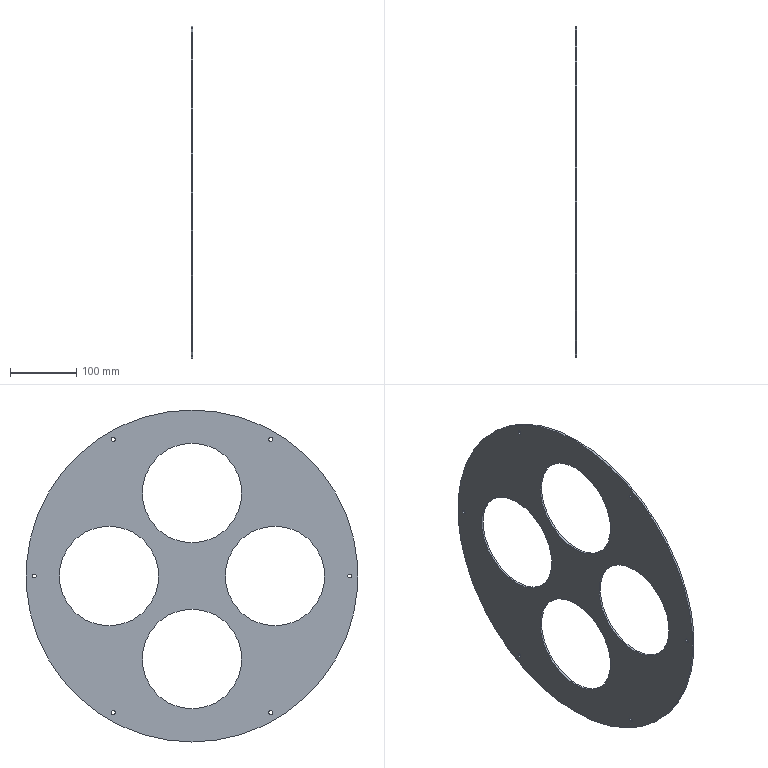Part | SolidWorks | features CirPattern 2, ICE 2, Extrusion 1 | 1 solid | 24 faces | box 3 x 500 x 500 mm | volume 376482 mm3 | cylinder 22 | plane 2 | commonest cylinder face diameters 6 x12 150 x8 500 x2
STEP:
#1=CARTESIAN_POINT('',(0.,118.75,208.681));
#2=VERTEX_POINT('',#1);
#3=CARTESIAN_POINT('',(0.,118.75,202.681));
#4=VERTEX_POINT('',#3);
#5=CARTESIAN_POINT('',(0.,118.75,205.681));
#6=DIRECTION('',(1.,0.,0.));
#7=DIRECTION('',(0.,0.,-1.));
#8=AXIS2_PLACEMENT_3D('',#5,#6,#7);
#9=CIRCLE('',#8,3.);
#10=EDGE_CURVE('',#2,#4,#9,.T.);
#11=ORIENTED_EDGE('',*,*,#10,.F.);
#12=CARTESIAN_POINT('',(3.,118.75,208.681));
#13=VERTEX_POINT('',#12);
#14=CARTESIAN_POINT('',(-17.,118.75,208.681));
#15=DIRECTION('',(1.,0.,0.));
#16=VECTOR('',#15,1000.);
#17=LINE('',#14,#16);
#18=EDGE_CURVE('',#2,#13,#17,.T.);
#19=ORIENTED_EDGE('',*,*,#18,.T.);
#20=CARTESIAN_POINT('',(3.,118.75,202.681));
#21=VERTEX_POINT('',#20);
#22=CARTESIAN_POINT('',(3.,118.75,205.681));
#23=DIRECTION('',(1.,0.,0.));
#24=DIRECTION('',(0.,-0.866,0.5));
#25=AXIS2_PLACEMENT_3D('',#22,#23,#24);
#26=CIRCLE('',#25,3.);
#27=EDGE_CURVE('',#13,#21,#26,.T.);
#28=ORIENTED_EDGE('',*,*,#27,.T.);
#29=CARTESIAN_POINT('',(-17.,118.75,202.681));
#30=DIRECTION('',(1.,0.,0.));
#31=VECTOR('',#30,1000.);
#32=LINE('',#29,#31);
#33=EDGE_CURVE('',#4,#21,#32,.T.);
#34=ORIENTED_EDGE('',*,*,#33,.F.);
#35=EDGE_LOOP('',(#11,#19,#28,#34));
#36=FACE_OUTER_BOUND('',#35,.T.);
#37=CARTESIAN_POINT('',(-17.,118.75,205.681));
#38=DIRECTION('',(1.,0.,0.));
#39=DIRECTION('',(0.,0.,-1.));
#40=AXIS2_PLACEMENT_3D('',#37,#38,#39);
#41=CYLINDRICAL_SURFACE('',#40,3.);
#42=ADVANCED_FACE('',(#36),#41,.F.);
#43=CARTESIAN_POINT('',(0.,237.5,3.));
#44=VERTEX_POINT('',#43);
#45=CARTESIAN_POINT('',(0.,237.5,-3.));
#46=VERTEX_POINT('',#45);
#47=CARTESIAN_POINT('',(0.,237.5,0.));
#48=DIRECTION('',(1.,0.,0.));
#49=DIRECTION('',(0.,0.,-1.));
#50=AXIS2_PLACEMENT_3D('',#47,#48,#49);
#51=CIRCLE('',#50,3.);
#52=EDGE_CURVE('',#44,#46,#51,.T.);
#53=ORIENTED_EDGE('',*,*,#52,.F.);
#54=CARTESIAN_POINT('',(3.,237.5,3.));
#55=VERTEX_POINT('',#54);
#56=CARTESIAN_POINT('',(-17.,237.5,3.));
#57=DIRECTION('',(1.,0.,0.));
#58=VECTOR('',#57,1000.);
#59=LINE('',#56,#58);
#60=EDGE_CURVE('',#44,#55,#59,.T.);
#61=ORIENTED_EDGE('',*,*,#60,.T.);
#62=CARTESIAN_POINT('',(3.,237.5,-3.));
#63=VERTEX_POINT('',#62);
#64=CARTESIAN_POINT('',(3.,237.5,0.));
#65=DIRECTION('',(1.,0.,0.));
#66=DIRECTION('',(0.,0.,1.));
#67=AXIS2_PLACEMENT_3D('',#64,#65,#66);
#68=CIRCLE('',#67,3.);
#69=EDGE_CURVE('',#55,#63,#68,.T.);
#70=ORIENTED_EDGE('',*,*,#69,.T.);
#71=CARTESIAN_POINT('',(-17.,237.5,-3.));
#72=DIRECTION('',(1.,0.,0.));
#73=VECTOR('',#72,1000.);
#74=LINE('',#71,#73);
#75=EDGE_CURVE('',#46,#63,#74,.T.);
#76=ORIENTED_EDGE('',*,*,#75,.F.);
#77=EDGE_LOOP('',(#53,#61,#70,#76));
#78=FACE_OUTER_BOUND('',#77,.T.);
#79=CARTESIAN_POINT('',(-17.,237.5,0.));
#80=DIRECTION('',(1.,0.,0.));
#81=DIRECTION('',(0.,0.,-1.));
#82=AXIS2_PLACEMENT_3D('',#79,#80,#81);
#83=CYLINDRICAL_SURFACE('',#82,3.);
#84=ADVANCED_FACE('',(#78),#83,.F.);
#85=CARTESIAN_POINT('',(0.,118.75,-202.681));
#86=VERTEX_POINT('',#85);
#87=CARTESIAN_POINT('',(0.,118.75,-208.681));
#88=VERTEX_POINT('',#87);
#89=CARTESIAN_POINT('',(0.,118.75,-205.681));
#90=DIRECTION('',(1.,0.,0.));
#91=DIRECTION('',(0.,0.,-1.));
#92=AXIS2_PLACEMENT_3D('',#89,#90,#91);
#93=CIRCLE('',#92,3.);
#94=EDGE_CURVE('',#86,#88,#93,.T.);
#95=ORIENTED_EDGE('',*,*,#94,.F.);
#96=CARTESIAN_POINT('',(3.,118.75,-202.681));
#97=VERTEX_POINT('',#96);
#98=CARTESIAN_POINT('',(-17.,118.75,-202.681));
#99=DIRECTION('',(1.,0.,0.));
#100=VECTOR('',#99,1000.);
#101=LINE('',#98,#100);
#102=EDGE_CURVE('',#86,#97,#101,.T.);
#103=ORIENTED_EDGE('',*,*,#102,.T.);
#104=CARTESIAN_POINT('',(3.,118.75,-208.681));
#105=VERTEX_POINT('',#104);
#106=CARTESIAN_POINT('',(3.,118.75,-205.681));
#107=DIRECTION('',(1.,0.,0.));
#108=DIRECTION('',(0.,0.866,0.5));
#109=AXIS2_PLACEMENT_3D('',#106,#107,#108);
#110=CIRCLE('',#109,3.);
#111=EDGE_CURVE('',#97,#105,#110,.T.);
#112=ORIENTED_EDGE('',*,*,#111,.T.);
#113=CARTESIAN_POINT('',(-17.,118.75,-208.681));
#114=DIRECTION('',(1.,0.,0.));
#115=VECTOR('',#114,1000.);
#116=LINE('',#113,#115);
#117=EDGE_CURVE('',#88,#105,#116,.T.);
#118=ORIENTED_EDGE('',*,*,#117,.F.);
#119=EDGE_LOOP('',(#95,#103,#112,#118));
#120=FACE_OUTER_BOUND('',#119,.T.);
#121=CARTESIAN_POINT('',(-17.,118.75,-205.681));
#122=DIRECTION('',(1.,0.,0.));
#123=DIRECTION('',(0.,0.,-1.));
#124=AXIS2_PLACEMENT_3D('',#121,#122,#123);
#125=CYLINDRICAL_SURFACE('',#124,3.);
#126=ADVANCED_FACE('',(#120),#125,.F.);
#127=CARTESIAN_POINT('',(0.,-118.75,-202.681));
#128=VERTEX_POINT('',#127);
#129=CARTESIAN_POINT('',(0.,-118.75,-208.681));
#130=VERTEX_POINT('',#129);
#131=CARTESIAN_POINT('',(0.,-118.75,-205.681));
#132=DIRECTION('',(1.,0.,0.));
#133=DIRECTION('',(0.,0.,-1.));
#134=AXIS2_PLACEMENT_3D('',#131,#132,#133);
#135=CIRCLE('',#134,3.);
#136=EDGE_CURVE('',#128,#130,#135,.T.);
#137=ORIENTED_EDGE('',*,*,#136,.F.);
#138=CARTESIAN_POINT('',(3.,-118.75,-202.681));
#139=VERTEX_POINT('',#138);
#140=CARTESIAN_POINT('',(-17.,-118.75,-202.681));
#141=DIRECTION('',(1.,0.,0.));
#142=VECTOR('',#141,1000.);
#143=LINE('',#140,#142);
#144=EDGE_CURVE('',#128,#139,#143,.T.);
#145=ORIENTED_EDGE('',*,*,#144,.T.);
#146=CARTESIAN_POINT('',(3.,-118.75,-208.681));
#147=VERTEX_POINT('',#146);
#148=CARTESIAN_POINT('',(3.,-118.75,-205.681));
#149=DIRECTION('',(1.,0.,0.));
#150=DIRECTION('',(0.,0.866,-0.5));
#151=AXIS2_PLACEMENT_3D('',#148,#149,#150);
#152=CIRCLE('',#151,3.);
#153=EDGE_CURVE('',#139,#147,#152,.T.);
#154=ORIENTED_EDGE('',*,*,#153,.T.);
#155=CARTESIAN_POINT('',(-17.,-118.75,-208.681));
#156=DIRECTION('',(1.,0.,0.));
#157=VECTOR('',#156,1000.);
#158=LINE('',#155,#157);
#159=EDGE_CURVE('',#130,#147,#158,.T.);
#160=ORIENTED_EDGE('',*,*,#159,.F.);
#161=EDGE_LOOP('',(#137,#145,#154,#160));
#162=FACE_OUTER_BOUND('',#161,.T.);
#163=CARTESIAN_POINT('',(-17.,-118.75,-205.681));
#164=DIRECTION('',(1.,0.,0.));
#165=DIRECTION('',(0.,0.,-1.));
#166=AXIS2_PLACEMENT_3D('',#163,#164,#165);
#167=CYLINDRICAL_SURFACE('',#166,3.);
#168=ADVANCED_FACE('',(#162),#167,.F.);
#169=CARTESIAN_POINT('',(0.,-118.75,208.681));
#170=VERTEX_POINT('',#169);
#171=CARTESIAN_POINT('',(0.,-118.75,202.681));
#172=VERTEX_POINT('',#171);
#173=CARTESIAN_POINT('',(0.,-118.75,205.681));
#174=DIRECTION('',(1.,0.,0.));
#175=DIRECTION('',(0.,0.,-1.));
#176=AXIS2_PLACEMENT_3D('',#173,#174,#175);
#177=CIRCLE('',#176,3.);
#178=EDGE_CURVE('',#170,#172,#177,.T.);
#179=ORIENTED_EDGE('',*,*,#178,.F.);
#180=CARTESIAN_POINT('',(3.,-118.75,208.681));
#181=VERTEX_POINT('',#180);
#182=CARTESIAN_POINT('',(-17.,-118.75,208.681));
#183=DIRECTION('',(1.,0.,0.));
#184=VECTOR('',#183,1000.);
#185=LINE('',#182,#184);
#186=EDGE_CURVE('',#170,#181,#185,.T.);
#187=ORIENTED_EDGE('',*,*,#186,.T.);
#188=CARTESIAN_POINT('',(3.,-118.75,202.681));
#189=VERTEX_POINT('',#188);
#190=CARTESIAN_POINT('',(3.,-118.75,205.681));
#191=DIRECTION('',(1.,0.,0.));
#192=DIRECTION('',(0.,-0.866,-0.5));
#193=AXIS2_PLACEMENT_3D('',#190,#191,#192);
#194=CIRCLE('',#193,3.);
#195=EDGE_CURVE('',#181,#189,#194,.T.);
#196=ORIENTED_EDGE('',*,*,#195,.T.);
#197=CARTESIAN_POINT('',(-17.,-118.75,202.681));
#198=DIRECTION('',(1.,0.,0.));
#199=VECTOR('',#198,1000.);
#200=LINE('',#197,#199);
#201=EDGE_CURVE('',#172,#189,#200,.T.);
#202=ORIENTED_EDGE('',*,*,#201,.F.);
#203=EDGE_LOOP('',(#179,#187,#196,#202));
#204=FACE_OUTER_BOUND('',#203,.T.);
#205=CARTESIAN_POINT('',(-17.,-118.75,205.681));
#206=DIRECTION('',(1.,0.,0.));
#207=DIRECTION('',(0.,0.,-1.));
#208=AXIS2_PLACEMENT_3D('',#205,#206,#207);
#209=CYLINDRICAL_SURFACE('',#208,3.);
#210=ADVANCED_FACE('',(#204),#209,.F.);
#211=CARTESIAN_POINT('',(0.,-237.5,3.));
#212=VERTEX_POINT('',#211);
#213=CARTESIAN_POINT('',(0.,-237.5,-3.));
#214=VERTEX_POINT('',#213);
#215=CARTESIAN_POINT('',(0.,-237.5,0.));
#216=DIRECTION('',(1.,0.,0.));
#217=DIRECTION('',(0.,0.,-1.));
#218=AXIS2_PLACEMENT_3D('',#215,#216,#217);
#219=CIRCLE('',#218,3.);
#220=EDGE_CURVE('',#212,#214,#219,.T.);
#221=ORIENTED_EDGE('',*,*,#220,.F.);
#222=CARTESIAN_POINT('',(3.,-237.5,3.));
#223=VERTEX_POINT('',#222);
#224=CARTESIAN_POINT('',(-17.,-237.5,3.));
#225=DIRECTION('',(1.,0.,0.));
#226=VECTOR('',#225,1000.);
#227=LINE('',#224,#226);
#228=EDGE_CURVE('',#212,#223,#227,.T.);
#229=ORIENTED_EDGE('',*,*,#228,.T.);
#230=CARTESIAN_POINT('',(3.,-237.5,-3.));
#231=VERTEX_POINT('',#230);
#232=CARTESIAN_POINT('',(3.,-237.5,0.));
#233=DIRECTION('',(1.,0.,0.));
#234=DIRECTION('',(0.,0.,-1.));
#235=AXIS2_PLACEMENT_3D('',#232,#233,#234);
#236=CIRCLE('',#235,3.);
#237=EDGE_CURVE('',#223,#231,#236,.T.);
#238=ORIENTED_EDGE('',*,*,#237,.T.);
#239=CARTESIAN_POINT('',(-17.,-237.5,-3.));
#240=DIRECTION('',(1.,0.,0.));
#241=VECTOR('',#240,1000.);
#242=LINE('',#239,#241);
#243=EDGE_CURVE('',#214,#231,#242,.T.);
#244=ORIENTED_EDGE('',*,*,#243,.F.);
#245=EDGE_LOOP('',(#221,#229,#238,#244));
#246=FACE_OUTER_BOUND('',#245,.T.);
#247=CARTESIAN_POINT('',(-17.,-237.5,0.));
#248=DIRECTION('',(1.,0.,0.));
#249=DIRECTION('',(0.,0.,-1.));
#250=AXIS2_PLACEMENT_3D('',#247,#248,#249);
#251=CYLINDRICAL_SURFACE('',#250,3.);
#252=ADVANCED_FACE('',(#246),#251,.F.);
#253=CARTESIAN_POINT('',(0.,0.,-50.));
#254=VERTEX_POINT('',#253);
#255=CARTESIAN_POINT('',(0.,0.,-200.));
#256=VERTEX_POINT('',#255);
#257=CARTESIAN_POINT('',(0.,0.,-125.));
#258=DIRECTION('',(1.,0.,0.));
#259=DIRECTION('',(0.,0.,-1.));
#260=AXIS2_PLACEMENT_3D('',#257,#258,#259);
#261=CIRCLE('',#260,75.);
#262=EDGE_CURVE('',#254,#256,#261,.T.);
#263=ORIENTED_EDGE('',*,*,#262,.F.);
#264=CARTESIAN_POINT('',(3.,0.,-50.));
#265=VERTEX_POINT('',#264);
#266=CARTESIAN_POINT('',(-7.,0.,-50.));
#267=DIRECTION('',(1.,0.,0.));
#268=VECTOR('',#267,1000.);
#269=LINE('',#266,#268);
#270=EDGE_CURVE('',#254,#265,#269,.T.);
#271=ORIENTED_EDGE('',*,*,#270,.T.);
#272=CARTESIAN_POINT('',(3.,0.,-200.));
#273=VERTEX_POINT('',#272);
#274=CARTESIAN_POINT('',(3.,0.,-125.));
#275=DIRECTION('',(1.,0.,0.));
#276=DIRECTION('',(0.,-1.,0.));
#277=AXIS2_PLACEMENT_3D('',#274,#275,#276);
#278=CIRCLE('',#277,75.);
#279=EDGE_CURVE('',#265,#273,#278,.T.);
#280=ORIENTED_EDGE('',*,*,#279,.T.);
#281=CARTESIAN_POINT('',(-7.,0.,-200.));
#282=DIRECTION('',(1.,0.,0.));
#283=VECTOR('',#282,1000.);
#284=LINE('',#281,#283);
#285=EDGE_CURVE('',#256,#273,#284,.T.);
#286=ORIENTED_EDGE('',*,*,#285,.F.);
#287=EDGE_LOOP('',(#263,#271,#280,#286));
#288=FACE_OUTER_BOUND('',#287,.T.);
#289=CARTESIAN_POINT('',(-7.,0.,-125.));
#290=DIRECTION('',(1.,0.,0.));
#291=DIRECTION('',(0.,0.,-1.));
#292=AXIS2_PLACEMENT_3D('',#289,#290,#291);
#293=CYLINDRICAL_SURFACE('',#292,75.);
#294=ADVANCED_FACE('',(#288),#293,.F.);
#295=CARTESIAN_POINT('',(0.,-125.,75.));
#296=VERTEX_POINT('',#295);
#297=CARTESIAN_POINT('',(0.,-125.,-75.));
#298=VERTEX_POINT('',#297);
#299=CARTESIAN_POINT('',(0.,-125.,0.));
#300=DIRECTION('',(1.,0.,0.));
#301=DIRECTION('',(0.,0.,-1.));
#302=AXIS2_PLACEMENT_3D('',#299,#300,#301);
#303=CIRCLE('',#302,75.);
#304=EDGE_CURVE('',#296,#298,#303,.T.);
#305=ORIENTED_EDGE('',*,*,#304,.F.);
#306=CARTESIAN_POINT('',(3.,-125.,75.));
#307=VERTEX_POINT('',#306);
#308=CARTESIAN_POINT('',(-7.,-125.,75.));
#309=DIRECTION('',(1.,0.,0.));
#310=VECTOR('',#309,1000.);
#311=LINE('',#308,#310);
#312=EDGE_CURVE('',#296,#307,#311,.T.);
#313=ORIENTED_EDGE('',*,*,#312,.T.);
#314=CARTESIAN_POINT('',(3.,-125.,-75.));
#315=VERTEX_POINT('',#314);
#316=CARTESIAN_POINT('',(3.,-125.,0.));
#317=DIRECTION('',(1.,0.,0.));
#318=DIRECTION('',(0.,0.,1.));
#319=AXIS2_PLACEMENT_3D('',#316,#317,#318);
#320=CIRCLE('',#319,75.);
#321=EDGE_CURVE('',#307,#315,#320,.T.);
#322=ORIENTED_EDGE('',*,*,#321,.T.);
#323=CARTESIAN_POINT('',(-7.,-125.,-75.));
#324=DIRECTION('',(1.,0.,0.));
#325=VECTOR('',#324,1000.);
#326=LINE('',#323,#325);
#327=EDGE_CURVE('',#298,#315,#326,.T.);
#328=ORIENTED_EDGE('',*,*,#327,.F.);
#329=EDGE_LOOP('',(#305,#313,#322,#328));
#330=FACE_OUTER_BOUND('',#329,.T.);
#331=CARTESIAN_POINT('',(-7.,-125.,0.));
#332=DIRECTION('',(1.,0.,0.));
#333=DIRECTION('',(0.,0.,-1.));
#334=AXIS2_PLACEMENT_3D('',#331,#332,#333);
#335=CYLINDRICAL_SURFACE('',#334,75.);
#336=ADVANCED_FACE('',(#330),#335,.F.);
#337=CARTESIAN_POINT('',(0.,0.,200.));
#338=VERTEX_POINT('',#337);
#339=CARTESIAN_POINT('',(0.,0.,50.));
#340=VERTEX_POINT('',#339);
#341=CARTESIAN_POINT('',(0.,0.,125.));
#342=DIRECTION('',(1.,0.,0.));
#343=DIRECTION('',(0.,0.,-1.));
#344=AXIS2_PLACEMENT_3D('',#341,#342,#343);
#345=CIRCLE('',#344,75.);
#346=EDGE_CURVE('',#338,#340,#345,.T.);
#347=ORIENTED_EDGE('',*,*,#346,.F.);
#348=CARTESIAN_POINT('',(3.,0.,200.));
#349=VERTEX_POINT('',#348);
#350=CARTESIAN_POINT('',(-7.,0.,200.));
#351=DIRECTION('',(1.,0.,0.));
#352=VECTOR('',#351,1000.);
#353=LINE('',#350,#352);
#354=EDGE_CURVE('',#338,#349,#353,.T.);
#355=ORIENTED_EDGE('',*,*,#354,.T.);
#356=CARTESIAN_POINT('',(3.,0.,50.));
#357=VERTEX_POINT('',#356);
#358=CARTESIAN_POINT('',(3.,0.,125.));
#359=DIRECTION('',(1.,0.,0.));
#360=DIRECTION('',(0.,1.,0.));
#361=AXIS2_PLACEMENT_3D('',#358,#359,#360);
#362=CIRCLE('',#361,75.);
#363=EDGE_CURVE('',#349,#357,#362,.T.);
#364=ORIENTED_EDGE('',*,*,#363,.T.);
#365=CARTESIAN_POINT('',(-7.,0.,50.));
#366=DIRECTION('',(1.,0.,0.));
#367=VECTOR('',#366,1000.);
#368=LINE('',#365,#367);
#369=EDGE_CURVE('',#340,#357,#368,.T.);
#370=ORIENTED_EDGE('',*,*,#369,.F.);
#371=EDGE_LOOP('',(#347,#355,#364,#370));
#372=FACE_OUTER_BOUND('',#371,.T.);
#373=CARTESIAN_POINT('',(-7.,0.,125.));
#374=DIRECTION('',(1.,0.,0.));
#375=DIRECTION('',(0.,0.,-1.));
#376=AXIS2_PLACEMENT_3D('',#373,#374,#375);
#377=CYLINDRICAL_SURFACE('',#376,75.);
#378=ADVANCED_FACE('',(#372),#377,.F.);
#379=CARTESIAN_POINT('',(0.,125.,75.));
#380=VERTEX_POINT('',#379);
#381=CARTESIAN_POINT('',(0.,125.,-75.));
#382=VERTEX_POINT('',#381);
#383=CARTESIAN_POINT('',(0.,125.,0.));
#384=DIRECTION('',(1.,0.,0.));
#385=DIRECTION('',(0.,0.,-1.));
#386=AXIS2_PLACEMENT_3D('',#383,#384,#385);
#387=CIRCLE('',#386,75.);
#388=EDGE_CURVE('',#380,#382,#387,.T.);
#389=ORIENTED_EDGE('',*,*,#388,.F.);
#390=CARTESIAN_POINT('',(3.,125.,75.));
#391=VERTEX_POINT('',#390);
#392=CARTESIAN_POINT('',(-7.,125.,75.));
#393=DIRECTION('',(1.,0.,0.));
#394=VECTOR('',#393,1000.);
#395=LINE('',#392,#394);
#396=EDGE_CURVE('',#380,#391,#395,.T.);
#397=ORIENTED_EDGE('',*,*,#396,.T.);
#398=CARTESIAN_POINT('',(3.,125.,-75.));
#399=VERTEX_POINT('',#398);
#400=CARTESIAN_POINT('',(3.,125.,0.));
#401=DIRECTION('',(1.,0.,0.));
#402=DIRECTION('',(0.,0.,-1.));
#403=AXIS2_PLACEMENT_3D('',#400,#401,#402);
#404=CIRCLE('',#403,75.);
#405=EDGE_CURVE('',#391,#399,#404,.T.);
#406=ORIENTED_EDGE('',*,*,#405,.T.);
#407=CARTESIAN_POINT('',(-7.,125.,-75.));
#408=DIRECTION('',(1.,0.,0.));
#409=VECTOR('',#408,1000.);
#410=LINE('',#407,#409);
#411=EDGE_CURVE('',#382,#399,#410,.T.);
#412=ORIENTED_EDGE('',*,*,#411,.F.);
#413=EDGE_LOOP('',(#389,#397,#406,#412));
#414=FACE_OUTER_BOUND('',#413,.T.);
#415=CARTESIAN_POINT('',(-7.,125.,0.));
#416=DIRECTION('',(1.,0.,0.));
#417=DIRECTION('',(0.,0.,-1.));
#418=AXIS2_PLACEMENT_3D('',#415,#416,#417);
#419=CYLINDRICAL_SURFACE('',#418,75.);
#420=ADVANCED_FACE('',(#414),#419,.F.);
#421=CARTESIAN_POINT('',(3.,0.,-250.));
#422=VERTEX_POINT('',#421);
#423=CARTESIAN_POINT('',(3.,0.,250.));
#424=VERTEX_POINT('',#423);
#425=CARTESIAN_POINT('',(3.,0.,0.));
#426=DIRECTION('',(1.,0.,0.));
#427=DIRECTION('',(0.,0.,-1.));
#428=AXIS2_PLACEMENT_3D('',#425,#426,#427);
#429=CIRCLE('',#428,250.);
#430=EDGE_CURVE('',#422,#424,#429,.T.);
#431=ORIENTED_EDGE('',*,*,#430,.F.);
#432=CARTESIAN_POINT('',(0.,0.,-250.));
#433=VERTEX_POINT('',#432);
#434=CARTESIAN_POINT('',(3.,0.,-250.));
#435=DIRECTION('',(-1.,0.,0.));
#436=VECTOR('',#435,1000.);
#437=LINE('',#434,#436);
#438=EDGE_CURVE('',#422,#433,#437,.T.);
#439=ORIENTED_EDGE('',*,*,#438,.T.);
#440=CARTESIAN_POINT('',(0.,0.,250.));
#441=VERTEX_POINT('',#440);
#442=CARTESIAN_POINT('',(0.,0.,0.));
#443=DIRECTION('',(1.,0.,0.));
#444=DIRECTION('',(0.,0.,-1.));
#445=AXIS2_PLACEMENT_3D('',#442,#443,#444);
#446=CIRCLE('',#445,250.);
#447=EDGE_CURVE('',#433,#441,#446,.T.);
#448=ORIENTED_EDGE('',*,*,#447,.T.);
#449=CARTESIAN_POINT('',(3.,0.,250.));
#450=DIRECTION('',(-1.,0.,0.));
#451=VECTOR('',#450,1000.);
#452=LINE('',#449,#451);
#453=EDGE_CURVE('',#424,#441,#452,.T.);
#454=ORIENTED_EDGE('',*,*,#453,.F.);
#455=EDGE_LOOP('',(#431,#439,#448,#454));
#456=FACE_OUTER_BOUND('',#455,.T.);
#457=CARTESIAN_POINT('',(3.,0.,0.));
#458=DIRECTION('',(-1.,0.,0.));
#459=DIRECTION('',(0.,0.,1.));
#460=AXIS2_PLACEMENT_3D('',#457,#458,#459);
#461=CYLINDRICAL_SURFACE('',#460,250.);
#462=ADVANCED_FACE('',(#456),#461,.T.);
#463=ORIENTED_EDGE('',*,*,#438,.F.);
#464=CARTESIAN_POINT('',(3.,0.,0.));
#465=DIRECTION('',(1.,0.,0.));
#466=DIRECTION('',(0.,0.,-1.));
#467=AXIS2_PLACEMENT_3D('',#464,#465,#466);
#468=CIRCLE('',#467,250.);
#469=EDGE_CURVE('',#424,#422,#468,.T.);
#470=ORIENTED_EDGE('',*,*,#469,.F.);
#471=ORIENTED_EDGE('',*,*,#453,.T.);
#472=CARTESIAN_POINT('',(0.,0.,0.));
#473=DIRECTION('',(1.,0.,0.));
#474=DIRECTION('',(0.,0.,-1.));
#475=AXIS2_PLACEMENT_3D('',#472,#473,#474);
#476=CIRCLE('',#475,250.);
#477=EDGE_CURVE('',#441,#433,#476,.T.);
#478=ORIENTED_EDGE('',*,*,#477,.T.);
#479=EDGE_LOOP('',(#463,#470,#471,#478));
#480=FACE_OUTER_BOUND('',#479,.T.);
#481=CARTESIAN_POINT('',(3.,0.,0.));
#482=DIRECTION('',(-1.,0.,0.));
#483=DIRECTION('',(0.,0.,1.));
#484=AXIS2_PLACEMENT_3D('',#481,#482,#483);
#485=CYLINDRICAL_SURFACE('',#484,250.);
#486=ADVANCED_FACE('',(#480),#485,.T.);
#487=CARTESIAN_POINT('',(3.,118.75,205.681));
#488=DIRECTION('',(1.,0.,0.));
#489=DIRECTION('',(0.,-0.866,0.5));
#490=AXIS2_PLACEMENT_3D('',#487,#488,#489);
#491=CIRCLE('',#490,3.);
#492=EDGE_CURVE('',#21,#13,#491,.T.);
#493=ORIENTED_EDGE('',*,*,#492,.F.);
#494=ORIENTED_EDGE('',*,*,#27,.F.);
#495=EDGE_LOOP('',(#493,#494));
#496=FACE_BOUND('',#495,.T.);
#497=CARTESIAN_POINT('',(3.,237.5,0.));
#498=DIRECTION('',(1.,0.,0.));
#499=DIRECTION('',(0.,0.,1.));
#500=AXIS2_PLACEMENT_3D('',#497,#498,#499);
#501=CIRCLE('',#500,3.);
#502=EDGE_CURVE('',#63,#55,#501,.T.);
#503=ORIENTED_EDGE('',*,*,#502,.F.);
#504=ORIENTED_EDGE('',*,*,#69,.F.);
#505=EDGE_LOOP('',(#503,#504));
#506=FACE_BOUND('',#505,.T.);
#507=CARTESIAN_POINT('',(3.,118.75,-205.681));
#508=DIRECTION('',(1.,0.,0.));
#509=DIRECTION('',(0.,0.866,0.5));
#510=AXIS2_PLACEMENT_3D('',#507,#508,#509);
#511=CIRCLE('',#510,3.);
#512=EDGE_CURVE('',#105,#97,#511,.T.);
#513=ORIENTED_EDGE('',*,*,#512,.F.);
#514=ORIENTED_EDGE('',*,*,#111,.F.);
#515=EDGE_LOOP('',(#513,#514));
#516=FACE_BOUND('',#515,.T.);
#517=CARTESIAN_POINT('',(3.,-118.75,-205.681));
#518=DIRECTION('',(1.,0.,0.));
#519=DIRECTION('',(0.,0.866,-0.5));
#520=AXIS2_PLACEMENT_3D('',#517,#518,#519);
#521=CIRCLE('',#520,3.);
#522=EDGE_CURVE('',#147,#139,#521,.T.);
#523=ORIENTED_EDGE('',*,*,#522,.F.);
#524=ORIENTED_EDGE('',*,*,#153,.F.);
#525=EDGE_LOOP('',(#523,#524));
#526=FACE_BOUND('',#525,.T.);
#527=CARTESIAN_POINT('',(3.,-118.75,205.681));
#528=DIRECTION('',(1.,0.,0.));
#529=DIRECTION('',(0.,-0.866,-0.5));
#530=AXIS2_PLACEMENT_3D('',#527,#528,#529);
#531=CIRCLE('',#530,3.);
#532=EDGE_CURVE('',#189,#181,#531,.T.);
#533=ORIENTED_EDGE('',*,*,#532,.F.);
#534=ORIENTED_EDGE('',*,*,#195,.F.);
#535=EDGE_LOOP('',(#533,#534));
#536=FACE_BOUND('',#535,.T.);
#537=CARTESIAN_POINT('',(3.,-237.5,0.));
#538=DIRECTION('',(1.,0.,0.));
#539=DIRECTION('',(0.,0.,-1.));
#540=AXIS2_PLACEMENT_3D('',#537,#538,#539);
#541=CIRCLE('',#540,3.);
#542=EDGE_CURVE('',#231,#223,#541,.T.);
#543=ORIENTED_EDGE('',*,*,#542,.F.);
#544=ORIENTED_EDGE('',*,*,#237,.F.);
#545=EDGE_LOOP('',(#543,#544));
#546=FACE_BOUND('',#545,.T.);
#547=CARTESIAN_POINT('',(3.,0.,-125.));
#548=DIRECTION('',(1.,0.,0.));
#549=DIRECTION('',(0.,-1.,0.));
#550=AXIS2_PLACEMENT_3D('',#547,#548,#549);
#551=CIRCLE('',#550,75.);
#552=EDGE_CURVE('',#273,#265,#551,.T.);
#553=ORIENTED_EDGE('',*,*,#552,.F.);
#554=ORIENTED_EDGE('',*,*,#279,.F.);
#555=EDGE_LOOP('',(#553,#554));
#556=FACE_BOUND('',#555,.T.);
#557=CARTESIAN_POINT('',(3.,-125.,0.));
#558=DIRECTION('',(1.,0.,0.));
#559=DIRECTION('',(0.,0.,1.));
#560=AXIS2_PLACEMENT_3D('',#557,#558,#559);
#561=CIRCLE('',#560,75.);
#562=EDGE_CURVE('',#315,#307,#561,.T.);
#563=ORIENTED_EDGE('',*,*,#562,.F.);
#564=ORIENTED_EDGE('',*,*,#321,.F.);
#565=EDGE_LOOP('',(#563,#564));
#566=FACE_BOUND('',#565,.T.);
#567=CARTESIAN_POINT('',(3.,0.,125.));
#568=DIRECTION('',(1.,0.,0.));
#569=DIRECTION('',(0.,1.,0.));
#570=AXIS2_PLACEMENT_3D('',#567,#568,#569);
#571=CIRCLE('',#570,75.);
#572=EDGE_CURVE('',#357,#349,#571,.T.);
#573=ORIENTED_EDGE('',*,*,#572,.F.);
#574=ORIENTED_EDGE('',*,*,#363,.F.);
#575=EDGE_LOOP('',(#573,#574));
#576=FACE_BOUND('',#575,.T.);
#577=CARTESIAN_POINT('',(3.,125.,0.));
#578=DIRECTION('',(1.,0.,0.));
#579=DIRECTION('',(0.,0.,-1.));
#580=AXIS2_PLACEMENT_3D('',#577,#578,#579);
#581=CIRCLE('',#580,75.);
#582=EDGE_CURVE('',#399,#391,#581,.T.);
#583=ORIENTED_EDGE('',*,*,#582,.F.);
#584=ORIENTED_EDGE('',*,*,#405,.F.);
#585=EDGE_LOOP('',(#583,#584));
#586=FACE_BOUND('',#585,.T.);
#587=ORIENTED_EDGE('',*,*,#469,.T.);
#588=ORIENTED_EDGE('',*,*,#430,.T.);
#589=EDGE_LOOP('',(#587,#588));
#590=FACE_OUTER_BOUND('',#589,.T.);
#591=CARTESIAN_POINT('',(3.,0.,0.));
#592=DIRECTION('',(1.,0.,0.));
#593=DIRECTION('',(0.,0.,-1.));
#594=AXIS2_PLACEMENT_3D('',#591,#592,#593);
#595=PLANE('',#594);
#596=ADVANCED_FACE('',(#496,#506,#516,#526,#536,#546,#556,#566,#576,#586,#590),#595,.T.);
#597=CARTESIAN_POINT('',(0.,118.75,205.681));
#598=DIRECTION('',(1.,0.,0.));
#599=DIRECTION('',(0.,0.,-1.));
#600=AXIS2_PLACEMENT_3D('',#597,#598,#599);
#601=CIRCLE('',#600,3.);
#602=EDGE_CURVE('',#4,#2,#601,.T.);
#603=ORIENTED_EDGE('',*,*,#602,.T.);
#604=ORIENTED_EDGE('',*,*,#10,.T.);
#605=EDGE_LOOP('',(#603,#604));
#606=FACE_BOUND('',#605,.T.);
#607=CARTESIAN_POINT('',(0.,237.5,0.));
#608=DIRECTION('',(1.,0.,0.));
#609=DIRECTION('',(0.,0.,-1.));
#610=AXIS2_PLACEMENT_3D('',#607,#608,#609);
#611=CIRCLE('',#610,3.);
#612=EDGE_CURVE('',#46,#44,#611,.T.);
#613=ORIENTED_EDGE('',*,*,#612,.T.);
#614=ORIENTED_EDGE('',*,*,#52,.T.);
#615=EDGE_LOOP('',(#613,#614));
#616=FACE_BOUND('',#615,.T.);
#617=CARTESIAN_POINT('',(0.,118.75,-205.681));
#618=DIRECTION('',(1.,0.,0.));
#619=DIRECTION('',(0.,0.,-1.));
#620=AXIS2_PLACEMENT_3D('',#617,#618,#619);
#621=CIRCLE('',#620,3.);
#622=EDGE_CURVE('',#88,#86,#621,.T.);
#623=ORIENTED_EDGE('',*,*,#622,.T.);
#624=ORIENTED_EDGE('',*,*,#94,.T.);
#625=EDGE_LOOP('',(#623,#624));
#626=FACE_BOUND('',#625,.T.);
#627=CARTESIAN_POINT('',(0.,-118.75,-205.681));
#628=DIRECTION('',(1.,0.,0.));
#629=DIRECTION('',(0.,0.,-1.));
#630=AXIS2_PLACEMENT_3D('',#627,#628,#629);
#631=CIRCLE('',#630,3.);
#632=EDGE_CURVE('',#130,#128,#631,.T.);
#633=ORIENTED_EDGE('',*,*,#632,.T.);
#634=ORIENTED_EDGE('',*,*,#136,.T.);
#635=EDGE_LOOP('',(#633,#634));
#636=FACE_BOUND('',#635,.T.);
#637=CARTESIAN_POINT('',(0.,-118.75,205.681));
#638=DIRECTION('',(1.,0.,0.));
#639=DIRECTION('',(0.,0.,-1.));
#640=AXIS2_PLACEMENT_3D('',#637,#638,#639);
#641=CIRCLE('',#640,3.);
#642=EDGE_CURVE('',#172,#170,#641,.T.);
#643=ORIENTED_EDGE('',*,*,#642,.T.);
#644=ORIENTED_EDGE('',*,*,#178,.T.);
#645=EDGE_LOOP('',(#643,#644));
#646=FACE_BOUND('',#645,.T.);
#647=CARTESIAN_POINT('',(0.,-237.5,0.));
#648=DIRECTION('',(1.,0.,0.));
#649=DIRECTION('',(0.,0.,-1.));
#650=AXIS2_PLACEMENT_3D('',#647,#648,#649);
#651=CIRCLE('',#650,3.);
#652=EDGE_CURVE('',#214,#212,#651,.T.);
#653=ORIENTED_EDGE('',*,*,#652,.T.);
#654=ORIENTED_EDGE('',*,*,#220,.T.);
#655=EDGE_LOOP('',(#653,#654));
#656=FACE_BOUND('',#655,.T.);
#657=CARTESIAN_POINT('',(0.,0.,-125.));
#658=DIRECTION('',(1.,0.,0.));
#659=DIRECTION('',(0.,0.,-1.));
#660=AXIS2_PLACEMENT_3D('',#657,#658,#659);
#661=CIRCLE('',#660,75.);
#662=EDGE_CURVE('',#256,#254,#661,.T.);
#663=ORIENTED_EDGE('',*,*,#662,.T.);
#664=ORIENTED_EDGE('',*,*,#262,.T.);
#665=EDGE_LOOP('',(#663,#664));
#666=FACE_BOUND('',#665,.T.);
#667=CARTESIAN_POINT('',(0.,-125.,0.));
#668=DIRECTION('',(1.,0.,0.));
#669=DIRECTION('',(0.,0.,-1.));
#670=AXIS2_PLACEMENT_3D('',#667,#668,#669);
#671=CIRCLE('',#670,75.);
#672=EDGE_CURVE('',#298,#296,#671,.T.);
#673=ORIENTED_EDGE('',*,*,#672,.T.);
#674=ORIENTED_EDGE('',*,*,#304,.T.);
#675=EDGE_LOOP('',(#673,#674));
#676=FACE_BOUND('',#675,.T.);
#677=CARTESIAN_POINT('',(0.,0.,125.));
#678=DIRECTION('',(1.,0.,0.));
#679=DIRECTION('',(0.,0.,-1.));
#680=AXIS2_PLACEMENT_3D('',#677,#678,#679);
#681=CIRCLE('',#680,75.);
#682=EDGE_CURVE('',#340,#338,#681,.T.);
#683=ORIENTED_EDGE('',*,*,#682,.T.);
#684=ORIENTED_EDGE('',*,*,#346,.T.);
#685=EDGE_LOOP('',(#683,#684));
#686=FACE_BOUND('',#685,.T.);
#687=CARTESIAN_POINT('',(0.,125.,0.));
#688=DIRECTION('',(1.,0.,0.));
#689=DIRECTION('',(0.,0.,-1.));
#690=AXIS2_PLACEMENT_3D('',#687,#688,#689);
#691=CIRCLE('',#690,75.);
#692=EDGE_CURVE('',#382,#380,#691,.T.);
#693=ORIENTED_EDGE('',*,*,#692,.T.);
#694=ORIENTED_EDGE('',*,*,#388,.T.);
#695=EDGE_LOOP('',(#693,#694));
#696=FACE_BOUND('',#695,.T.);
#697=ORIENTED_EDGE('',*,*,#477,.F.);
#698=ORIENTED_EDGE('',*,*,#447,.F.);
#699=EDGE_LOOP('',(#697,#698));
#700=FACE_OUTER_BOUND('',#699,.T.);
#701=CARTESIAN_POINT('',(0.,0.,0.));
#702=DIRECTION('',(1.,0.,0.));
#703=DIRECTION('',(0.,0.,-1.));
#704=AXIS2_PLACEMENT_3D('',#701,#702,#703);
#705=PLANE('',#704);
#706=ADVANCED_FACE('',(#606,#616,#626,#636,#646,#656,#666,#676,#686,#696,#700),#705,.F.);
#707=ORIENTED_EDGE('',*,*,#396,.F.);
#708=ORIENTED_EDGE('',*,*,#692,.F.);
#709=ORIENTED_EDGE('',*,*,#411,.T.);
#710=ORIENTED_EDGE('',*,*,#582,.T.);
#711=EDGE_LOOP('',(#707,#708,#709,#710));
#712=FACE_OUTER_BOUND('',#711,.T.);
#713=CARTESIAN_POINT('',(-7.,125.,0.));
#714=DIRECTION('',(1.,0.,0.));
#715=DIRECTION('',(0.,0.,-1.));
#716=AXIS2_PLACEMENT_3D('',#713,#714,#715);
#717=CYLINDRICAL_SURFACE('',#716,75.);
#718=ADVANCED_FACE('',(#712),#717,.F.);
#719=ORIENTED_EDGE('',*,*,#354,.F.);
#720=ORIENTED_EDGE('',*,*,#682,.F.);
#721=ORIENTED_EDGE('',*,*,#369,.T.);
#722=ORIENTED_EDGE('',*,*,#572,.T.);
#723=EDGE_LOOP('',(#719,#720,#721,#722));
#724=FACE_OUTER_BOUND('',#723,.T.);
#725=CARTESIAN_POINT('',(-7.,0.,125.));
#726=DIRECTION('',(1.,0.,0.));
#727=DIRECTION('',(0.,0.,-1.));
#728=AXIS2_PLACEMENT_3D('',#725,#726,#727);
#729=CYLINDRICAL_SURFACE('',#728,75.);
#730=ADVANCED_FACE('',(#724),#729,.F.);
#731=ORIENTED_EDGE('',*,*,#312,.F.);
#732=ORIENTED_EDGE('',*,*,#672,.F.);
#733=ORIENTED_EDGE('',*,*,#327,.T.);
#734=ORIENTED_EDGE('',*,*,#562,.T.);
#735=EDGE_LOOP('',(#731,#732,#733,#734));
#736=FACE_OUTER_BOUND('',#735,.T.);
#737=CARTESIAN_POINT('',(-7.,-125.,0.));
#738=DIRECTION('',(1.,0.,0.));
#739=DIRECTION('',(0.,0.,-1.));
#740=AXIS2_PLACEMENT_3D('',#737,#738,#739);
#741=CYLINDRICAL_SURFACE('',#740,75.);
#742=ADVANCED_FACE('',(#736),#741,.F.);
#743=ORIENTED_EDGE('',*,*,#270,.F.);
#744=ORIENTED_EDGE('',*,*,#662,.F.);
#745=ORIENTED_EDGE('',*,*,#285,.T.);
#746=ORIENTED_EDGE('',*,*,#552,.T.);
#747=EDGE_LOOP('',(#743,#744,#745,#746));
#748=FACE_OUTER_BOUND('',#747,.T.);
#749=CARTESIAN_POINT('',(-7.,0.,-125.));
#750=DIRECTION('',(1.,0.,0.));
#751=DIRECTION('',(0.,0.,-1.));
#752=AXIS2_PLACEMENT_3D('',#749,#750,#751);
#753=CYLINDRICAL_SURFACE('',#752,75.);
#754=ADVANCED_FACE('',(#748),#753,.F.);
#755=ORIENTED_EDGE('',*,*,#228,.F.);
#756=ORIENTED_EDGE('',*,*,#652,.F.);
#757=ORIENTED_EDGE('',*,*,#243,.T.);
#758=ORIENTED_EDGE('',*,*,#542,.T.);
#759=EDGE_LOOP('',(#755,#756,#757,#758));
#760=FACE_OUTER_BOUND('',#759,.T.);
#761=CARTESIAN_POINT('',(-17.,-237.5,0.));
#762=DIRECTION('',(1.,0.,0.));
#763=DIRECTION('',(0.,0.,-1.));
#764=AXIS2_PLACEMENT_3D('',#761,#762,#763);
#765=CYLINDRICAL_SURFACE('',#764,3.);
#766=ADVANCED_FACE('',(#760),#765,.F.);
#767=ORIENTED_EDGE('',*,*,#186,.F.);
#768=ORIENTED_EDGE('',*,*,#642,.F.);
#769=ORIENTED_EDGE('',*,*,#201,.T.);
#770=ORIENTED_EDGE('',*,*,#532,.T.);
#771=EDGE_LOOP('',(#767,#768,#769,#770));
#772=FACE_OUTER_BOUND('',#771,.T.);
#773=CARTESIAN_POINT('',(-17.,-118.75,205.681));
#774=DIRECTION('',(1.,0.,0.));
#775=DIRECTION('',(0.,0.,-1.));
#776=AXIS2_PLACEMENT_3D('',#773,#774,#775);
#777=CYLINDRICAL_SURFACE('',#776,3.);
#778=ADVANCED_FACE('',(#772),#777,.F.);
#779=ORIENTED_EDGE('',*,*,#144,.F.);
#780=ORIENTED_EDGE('',*,*,#632,.F.);
#781=ORIENTED_EDGE('',*,*,#159,.T.);
#782=ORIENTED_EDGE('',*,*,#522,.T.);
#783=EDGE_LOOP('',(#779,#780,#781,#782));
#784=FACE_OUTER_BOUND('',#783,.T.);
#785=CARTESIAN_POINT('',(-17.,-118.75,-205.681));
#786=DIRECTION('',(1.,0.,0.));
#787=DIRECTION('',(0.,0.,-1.));
#788=AXIS2_PLACEMENT_3D('',#785,#786,#787);
#789=CYLINDRICAL_SURFACE('',#788,3.);
#790=ADVANCED_FACE('',(#784),#789,.F.);
#791=ORIENTED_EDGE('',*,*,#102,.F.);
#792=ORIENTED_EDGE('',*,*,#622,.F.);
#793=ORIENTED_EDGE('',*,*,#117,.T.);
#794=ORIENTED_EDGE('',*,*,#512,.T.);
#795=EDGE_LOOP('',(#791,#792,#793,#794));
#796=FACE_OUTER_BOUND('',#795,.T.);
#797=CARTESIAN_POINT('',(-17.,118.75,-205.681));
#798=DIRECTION('',(1.,0.,0.));
#799=DIRECTION('',(0.,0.,-1.));
#800=AXIS2_PLACEMENT_3D('',#797,#798,#799);
#801=CYLINDRICAL_SURFACE('',#800,3.);
#802=ADVANCED_FACE('',(#796),#801,.F.);
#803=ORIENTED_EDGE('',*,*,#60,.F.);
#804=ORIENTED_EDGE('',*,*,#612,.F.);
#805=ORIENTED_EDGE('',*,*,#75,.T.);
#806=ORIENTED_EDGE('',*,*,#502,.T.);
#807=EDGE_LOOP('',(#803,#804,#805,#806));
#808=FACE_OUTER_BOUND('',#807,.T.);
#809=CARTESIAN_POINT('',(-17.,237.5,0.));
#810=DIRECTION('',(1.,0.,0.));
#811=DIRECTION('',(0.,0.,-1.));
#812=AXIS2_PLACEMENT_3D('',#809,#810,#811);
#813=CYLINDRICAL_SURFACE('',#812,3.);
#814=ADVANCED_FACE('',(#808),#813,.F.);
#815=ORIENTED_EDGE('',*,*,#18,.F.);
#816=ORIENTED_EDGE('',*,*,#602,.F.);
#817=ORIENTED_EDGE('',*,*,#33,.T.);
#818=ORIENTED_EDGE('',*,*,#492,.T.);
#819=EDGE_LOOP('',(#815,#816,#817,#818));
#820=FACE_OUTER_BOUND('',#819,.T.);
#821=CARTESIAN_POINT('',(-17.,118.75,205.681));
#822=DIRECTION('',(1.,0.,0.));
#823=DIRECTION('',(0.,0.,-1.));
#824=AXIS2_PLACEMENT_3D('',#821,#822,#823);
#825=CYLINDRICAL_SURFACE('',#824,3.);
#826=ADVANCED_FACE('',(#820),#825,.F.);
#827=CLOSED_SHELL('',(#42,#84,#126,#168,#210,#252,#294,#336,#378,#420,#462,#486,#596,#706,#718,#730,#742,#754,#766,#778,#790,#802,#814,#826));
#828=MANIFOLD_SOLID_BREP('',#827);
#829=CARTESIAN_POINT('',(0.,0.,0.));
#830=DIRECTION('',(0.,0.,1.));
#831=DIRECTION('',(1.,0.,0.));
#832=AXIS2_PLACEMENT_3D('',#829,#830,#831);
#833=(LENGTH_UNIT()NAMED_UNIT(*)SI_UNIT(.MILLI.,.METRE.));
#834=UNCERTAINTY_MEASURE_WITH_UNIT(LENGTH_MEASURE(0.00001),#833,'','');
#835=(NAMED_UNIT(*)PLANE_ANGLE_UNIT()SI_UNIT($,.RADIAN.));
#836=(NAMED_UNIT(*)SI_UNIT($,.STERADIAN.)SOLID_ANGLE_UNIT());
#837=(GEOMETRIC_REPRESENTATION_CONTEXT(3)GLOBAL_UNCERTAINTY_ASSIGNED_CONTEXT((#834))GLOBAL_UNIT_ASSIGNED_CONTEXT((#833,#835,#836))REPRESENTATION_CONTEXT('',''));
#838=ADVANCED_BREP_SHAPE_REPRESENTATION('',(#828,#832),#837);